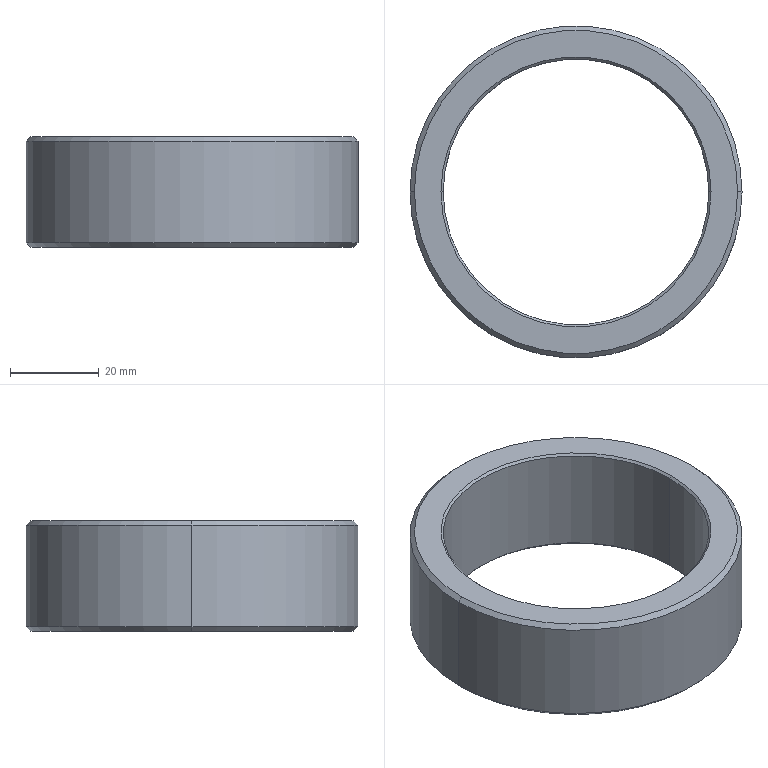Part | SolidWorks | features MBimport 1 | 1 solid | 14 faces | box 75 x 75 x 25 mm | volume 39480 mm3 | cone 8 | cylinder 4 | plane 2 | commonest cylinder face diameters 60 x2 75 x2
STEP:
#1=CARTESIAN_POINT('',(-36.5,0.,-28.514));
#2=VERTEX_POINT('',#1);
#3=CARTESIAN_POINT('',(-37.5,0.,-27.514));
#4=VERTEX_POINT('',#3);
#5=CARTESIAN_POINT('',(-37.5,0.,-27.514));
#6=DIRECTION('',(-0.7071,0.,0.7071));
#7=VECTOR('',#6,1000.);
#8=LINE('',#5,#7);
#9=EDGE_CURVE('',#2,#4,#8,.T.);
#10=ORIENTED_EDGE('',*,*,#9,.F.);
#11=CARTESIAN_POINT('',(36.5,0.,-28.514));
#12=VERTEX_POINT('',#11);
#13=CARTESIAN_POINT('',(0.,0.,-28.514));
#14=DIRECTION('',(0.,0.,-1.));
#15=DIRECTION('',(1.,0.,0.));
#16=AXIS2_PLACEMENT_3D('',#13,#14,#15);
#17=CIRCLE('',#16,36.5);
#18=EDGE_CURVE('',#12,#2,#17,.T.);
#19=ORIENTED_EDGE('',*,*,#18,.F.);
#20=CARTESIAN_POINT('',(37.5,0.,-27.514));
#21=VERTEX_POINT('',#20);
#22=CARTESIAN_POINT('',(37.5,0.,-27.514));
#23=DIRECTION('',(0.7071,0.,0.7071));
#24=VECTOR('',#23,1000.);
#25=LINE('',#22,#24);
#26=EDGE_CURVE('',#12,#21,#25,.T.);
#27=ORIENTED_EDGE('',*,*,#26,.T.);
#28=CARTESIAN_POINT('',(0.,0.,-27.514));
#29=DIRECTION('',(0.,0.,1.));
#30=DIRECTION('',(1.,0.,0.));
#31=AXIS2_PLACEMENT_3D('',#28,#29,#30);
#32=CIRCLE('',#31,37.5);
#33=EDGE_CURVE('',#4,#21,#32,.T.);
#34=ORIENTED_EDGE('',*,*,#33,.F.);
#35=EDGE_LOOP('',(#10,#19,#27,#34));
#36=FACE_OUTER_BOUND('',#35,.T.);
#37=CARTESIAN_POINT('',(0.,0.,-27.514));
#38=DIRECTION('',(0.,0.,1.));
#39=DIRECTION('',(1.,0.,0.));
#40=AXIS2_PLACEMENT_3D('',#37,#38,#39);
#41=CONICAL_SURFACE('',#40,37.5,0.7854);
#42=ADVANCED_FACE('',(#36),#41,.T.);
#43=CARTESIAN_POINT('',(30.,0.,-28.014));
#44=VERTEX_POINT('',#43);
#45=CARTESIAN_POINT('',(30.5,0.,-28.514));
#46=VERTEX_POINT('',#45);
#47=CARTESIAN_POINT('',(30.5,0.,-28.514));
#48=DIRECTION('',(0.7071,0.,-0.7071));
#49=VECTOR('',#48,1000.);
#50=LINE('',#47,#49);
#51=EDGE_CURVE('',#44,#46,#50,.T.);
#52=ORIENTED_EDGE('',*,*,#51,.F.);
#53=CARTESIAN_POINT('',(-30.,0.,-28.014));
#54=VERTEX_POINT('',#53);
#55=CARTESIAN_POINT('',(0.,0.,-28.014));
#56=DIRECTION('',(0.,0.,-1.));
#57=DIRECTION('',(1.,0.,0.));
#58=AXIS2_PLACEMENT_3D('',#55,#56,#57);
#59=CIRCLE('',#58,30.);
#60=EDGE_CURVE('',#54,#44,#59,.T.);
#61=ORIENTED_EDGE('',*,*,#60,.F.);
#62=CARTESIAN_POINT('',(-30.5,0.,-28.514));
#63=VERTEX_POINT('',#62);
#64=CARTESIAN_POINT('',(-30.5,0.,-28.514));
#65=DIRECTION('',(-0.7071,0.,-0.7071));
#66=VECTOR('',#65,1000.);
#67=LINE('',#64,#66);
#68=EDGE_CURVE('',#54,#63,#67,.T.);
#69=ORIENTED_EDGE('',*,*,#68,.T.);
#70=CARTESIAN_POINT('',(0.,0.,-28.514));
#71=DIRECTION('',(0.,0.,1.));
#72=DIRECTION('',(1.,0.,0.));
#73=AXIS2_PLACEMENT_3D('',#70,#71,#72);
#74=CIRCLE('',#73,30.5);
#75=EDGE_CURVE('',#46,#63,#74,.T.);
#76=ORIENTED_EDGE('',*,*,#75,.F.);
#77=EDGE_LOOP('',(#52,#61,#69,#76));
#78=FACE_OUTER_BOUND('',#77,.T.);
#79=CARTESIAN_POINT('',(0.,0.,-28.514));
#80=DIRECTION('',(0.,0.,-1.));
#81=DIRECTION('',(-1.,0.,0.));
#82=AXIS2_PLACEMENT_3D('',#79,#80,#81);
#83=CONICAL_SURFACE('',#82,30.5,0.7854);
#84=ADVANCED_FACE('',(#78),#83,.F.);
#85=CARTESIAN_POINT('',(36.5,0.,-3.514));
#86=VERTEX_POINT('',#85);
#87=CARTESIAN_POINT('',(37.5,0.,-4.514));
#88=VERTEX_POINT('',#87);
#89=CARTESIAN_POINT('',(36.5,0.,-3.514));
#90=DIRECTION('',(0.7071,0.,-0.7071));
#91=VECTOR('',#90,1000.);
#92=LINE('',#89,#91);
#93=EDGE_CURVE('',#86,#88,#92,.T.);
#94=ORIENTED_EDGE('',*,*,#93,.F.);
#95=CARTESIAN_POINT('',(-36.5,0.,-3.514));
#96=VERTEX_POINT('',#95);
#97=CARTESIAN_POINT('',(0.,0.,-3.514));
#98=DIRECTION('',(0.,0.,1.));
#99=DIRECTION('',(-1.,0.,0.));
#100=AXIS2_PLACEMENT_3D('',#97,#98,#99);
#101=CIRCLE('',#100,36.5);
#102=EDGE_CURVE('',#96,#86,#101,.T.);
#103=ORIENTED_EDGE('',*,*,#102,.F.);
#104=CARTESIAN_POINT('',(-37.5,0.,-4.514));
#105=VERTEX_POINT('',#104);
#106=CARTESIAN_POINT('',(-36.5,0.,-3.514));
#107=DIRECTION('',(-0.7071,0.,-0.7071));
#108=VECTOR('',#107,1000.);
#109=LINE('',#106,#108);
#110=EDGE_CURVE('',#96,#105,#109,.T.);
#111=ORIENTED_EDGE('',*,*,#110,.T.);
#112=CARTESIAN_POINT('',(0.,0.,-4.514));
#113=DIRECTION('',(0.,0.,-1.));
#114=DIRECTION('',(-1.,0.,0.));
#115=AXIS2_PLACEMENT_3D('',#112,#113,#114);
#116=CIRCLE('',#115,37.5);
#117=EDGE_CURVE('',#88,#105,#116,.T.);
#118=ORIENTED_EDGE('',*,*,#117,.F.);
#119=EDGE_LOOP('',(#94,#103,#111,#118));
#120=FACE_OUTER_BOUND('',#119,.T.);
#121=CARTESIAN_POINT('',(0.,0.,-3.514));
#122=DIRECTION('',(0.,0.,-1.));
#123=DIRECTION('',(-1.,0.,0.));
#124=AXIS2_PLACEMENT_3D('',#121,#122,#123);
#125=CONICAL_SURFACE('',#124,36.5,0.7854);
#126=ADVANCED_FACE('',(#120),#125,.T.);
#127=CARTESIAN_POINT('',(-30.,0.,-4.014));
#128=VERTEX_POINT('',#127);
#129=CARTESIAN_POINT('',(-30.5,0.,-3.514));
#130=VERTEX_POINT('',#129);
#131=CARTESIAN_POINT('',(-30.,0.,-4.014));
#132=DIRECTION('',(-0.7071,0.,0.7071));
#133=VECTOR('',#132,1000.);
#134=LINE('',#131,#133);
#135=EDGE_CURVE('',#128,#130,#134,.T.);
#136=ORIENTED_EDGE('',*,*,#135,.F.);
#137=CARTESIAN_POINT('',(30.,0.,-4.014));
#138=VERTEX_POINT('',#137);
#139=CARTESIAN_POINT('',(0.,0.,-4.014));
#140=DIRECTION('',(0.,0.,1.));
#141=DIRECTION('',(-1.,0.,0.));
#142=AXIS2_PLACEMENT_3D('',#139,#140,#141);
#143=CIRCLE('',#142,30.);
#144=EDGE_CURVE('',#138,#128,#143,.T.);
#145=ORIENTED_EDGE('',*,*,#144,.F.);
#146=CARTESIAN_POINT('',(30.5,0.,-3.514));
#147=VERTEX_POINT('',#146);
#148=CARTESIAN_POINT('',(30.,0.,-4.014));
#149=DIRECTION('',(0.7071,0.,0.7071));
#150=VECTOR('',#149,1000.);
#151=LINE('',#148,#150);
#152=EDGE_CURVE('',#138,#147,#151,.T.);
#153=ORIENTED_EDGE('',*,*,#152,.T.);
#154=CARTESIAN_POINT('',(0.,0.,-3.514));
#155=DIRECTION('',(0.,0.,-1.));
#156=DIRECTION('',(-1.,0.,0.));
#157=AXIS2_PLACEMENT_3D('',#154,#155,#156);
#158=CIRCLE('',#157,30.5);
#159=EDGE_CURVE('',#130,#147,#158,.T.);
#160=ORIENTED_EDGE('',*,*,#159,.F.);
#161=EDGE_LOOP('',(#136,#145,#153,#160));
#162=FACE_OUTER_BOUND('',#161,.T.);
#163=CARTESIAN_POINT('',(0.,0.,-4.014));
#164=DIRECTION('',(0.,0.,1.));
#165=DIRECTION('',(1.,0.,0.));
#166=AXIS2_PLACEMENT_3D('',#163,#164,#165);
#167=CONICAL_SURFACE('',#166,30.,0.7854);
#168=ADVANCED_FACE('',(#162),#167,.F.);
#169=CARTESIAN_POINT('',(0.,0.,-28.514));
#170=DIRECTION('',(0.,0.,1.));
#171=DIRECTION('',(1.,0.,0.));
#172=AXIS2_PLACEMENT_3D('',#169,#170,#171);
#173=CIRCLE('',#172,30.5);
#174=EDGE_CURVE('',#63,#46,#173,.T.);
#175=ORIENTED_EDGE('',*,*,#174,.T.);
#176=ORIENTED_EDGE('',*,*,#75,.T.);
#177=EDGE_LOOP('',(#175,#176));
#178=FACE_BOUND('',#177,.T.);
#179=ORIENTED_EDGE('',*,*,#18,.T.);
#180=CARTESIAN_POINT('',(0.,0.,-28.514));
#181=DIRECTION('',(0.,0.,-1.));
#182=DIRECTION('',(1.,0.,0.));
#183=AXIS2_PLACEMENT_3D('',#180,#181,#182);
#184=CIRCLE('',#183,36.5);
#185=EDGE_CURVE('',#2,#12,#184,.T.);
#186=ORIENTED_EDGE('',*,*,#185,.T.);
#187=EDGE_LOOP('',(#179,#186));
#188=FACE_OUTER_BOUND('',#187,.T.);
#189=CARTESIAN_POINT('',(-37.5,0.,-28.514));
#190=DIRECTION('',(0.,0.,1.));
#191=DIRECTION('',(1.,0.,0.));
#192=AXIS2_PLACEMENT_3D('',#189,#190,#191);
#193=PLANE('',#192);
#194=ADVANCED_FACE('',(#178,#188),#193,.F.);
#195=CARTESIAN_POINT('',(-30.,0.,0.));
#196=DIRECTION('',(0.,0.,1.));
#197=VECTOR('',#196,1000.);
#198=LINE('',#195,#197);
#199=EDGE_CURVE('',#54,#128,#198,.T.);
#200=ORIENTED_EDGE('',*,*,#199,.F.);
#201=ORIENTED_EDGE('',*,*,#60,.T.);
#202=CARTESIAN_POINT('',(30.,0.,0.));
#203=DIRECTION('',(0.,0.,1.));
#204=VECTOR('',#203,1000.);
#205=LINE('',#202,#204);
#206=EDGE_CURVE('',#44,#138,#205,.T.);
#207=ORIENTED_EDGE('',*,*,#206,.T.);
#208=ORIENTED_EDGE('',*,*,#144,.T.);
#209=EDGE_LOOP('',(#200,#201,#207,#208));
#210=FACE_OUTER_BOUND('',#209,.T.);
#211=CARTESIAN_POINT('',(0.,0.,0.));
#212=DIRECTION('',(0.,0.,1.));
#213=DIRECTION('',(1.,0.,0.));
#214=AXIS2_PLACEMENT_3D('',#211,#212,#213);
#215=CYLINDRICAL_SURFACE('',#214,30.);
#216=ADVANCED_FACE('',(#210),#215,.F.);
#217=CARTESIAN_POINT('',(0.,0.,-3.514));
#218=DIRECTION('',(0.,0.,-1.));
#219=DIRECTION('',(-1.,0.,0.));
#220=AXIS2_PLACEMENT_3D('',#217,#218,#219);
#221=CIRCLE('',#220,30.5);
#222=EDGE_CURVE('',#147,#130,#221,.T.);
#223=ORIENTED_EDGE('',*,*,#222,.T.);
#224=ORIENTED_EDGE('',*,*,#159,.T.);
#225=EDGE_LOOP('',(#223,#224));
#226=FACE_BOUND('',#225,.T.);
#227=ORIENTED_EDGE('',*,*,#102,.T.);
#228=CARTESIAN_POINT('',(0.,0.,-3.514));
#229=DIRECTION('',(0.,0.,1.));
#230=DIRECTION('',(-1.,0.,0.));
#231=AXIS2_PLACEMENT_3D('',#228,#229,#230);
#232=CIRCLE('',#231,36.5);
#233=EDGE_CURVE('',#86,#96,#232,.T.);
#234=ORIENTED_EDGE('',*,*,#233,.T.);
#235=EDGE_LOOP('',(#227,#234));
#236=FACE_OUTER_BOUND('',#235,.T.);
#237=CARTESIAN_POINT('',(-37.5,0.,-3.514));
#238=DIRECTION('',(0.,0.,-1.));
#239=DIRECTION('',(0.,-1.,0.));
#240=AXIS2_PLACEMENT_3D('',#237,#238,#239);
#241=PLANE('',#240);
#242=ADVANCED_FACE('',(#226,#236),#241,.F.);
#243=CARTESIAN_POINT('',(-37.5,0.,0.));
#244=DIRECTION('',(0.,0.,1.));
#245=VECTOR('',#244,1000.);
#246=LINE('',#243,#245);
#247=EDGE_CURVE('',#4,#105,#246,.T.);
#248=ORIENTED_EDGE('',*,*,#247,.F.);
#249=ORIENTED_EDGE('',*,*,#33,.T.);
#250=CARTESIAN_POINT('',(37.5,0.,0.));
#251=DIRECTION('',(0.,0.,1.));
#252=VECTOR('',#251,1000.);
#253=LINE('',#250,#252);
#254=EDGE_CURVE('',#21,#88,#253,.T.);
#255=ORIENTED_EDGE('',*,*,#254,.T.);
#256=ORIENTED_EDGE('',*,*,#117,.T.);
#257=EDGE_LOOP('',(#248,#249,#255,#256));
#258=FACE_OUTER_BOUND('',#257,.T.);
#259=CARTESIAN_POINT('',(0.,0.,0.));
#260=DIRECTION('',(0.,0.,1.));
#261=DIRECTION('',(1.,0.,0.));
#262=AXIS2_PLACEMENT_3D('',#259,#260,#261);
#263=CYLINDRICAL_SURFACE('',#262,37.5);
#264=ADVANCED_FACE('',(#258),#263,.T.);
#265=CARTESIAN_POINT('',(0.,0.,-27.514));
#266=DIRECTION('',(0.,0.,1.));
#267=DIRECTION('',(1.,0.,0.));
#268=AXIS2_PLACEMENT_3D('',#265,#266,#267);
#269=CIRCLE('',#268,37.5);
#270=EDGE_CURVE('',#21,#4,#269,.T.);
#271=ORIENTED_EDGE('',*,*,#270,.T.);
#272=ORIENTED_EDGE('',*,*,#247,.T.);
#273=CARTESIAN_POINT('',(0.,0.,-4.514));
#274=DIRECTION('',(0.,0.,-1.));
#275=DIRECTION('',(-1.,0.,0.));
#276=AXIS2_PLACEMENT_3D('',#273,#274,#275);
#277=CIRCLE('',#276,37.5);
#278=EDGE_CURVE('',#105,#88,#277,.T.);
#279=ORIENTED_EDGE('',*,*,#278,.T.);
#280=ORIENTED_EDGE('',*,*,#254,.F.);
#281=EDGE_LOOP('',(#271,#272,#279,#280));
#282=FACE_OUTER_BOUND('',#281,.T.);
#283=CARTESIAN_POINT('',(0.,0.,0.));
#284=DIRECTION('',(0.,0.,1.));
#285=DIRECTION('',(1.,0.,0.));
#286=AXIS2_PLACEMENT_3D('',#283,#284,#285);
#287=CYLINDRICAL_SURFACE('',#286,37.5);
#288=ADVANCED_FACE('',(#282),#287,.T.);
#289=CARTESIAN_POINT('',(0.,0.,-28.014));
#290=DIRECTION('',(0.,0.,-1.));
#291=DIRECTION('',(1.,0.,0.));
#292=AXIS2_PLACEMENT_3D('',#289,#290,#291);
#293=CIRCLE('',#292,30.);
#294=EDGE_CURVE('',#44,#54,#293,.T.);
#295=ORIENTED_EDGE('',*,*,#294,.T.);
#296=ORIENTED_EDGE('',*,*,#199,.T.);
#297=CARTESIAN_POINT('',(0.,0.,-4.014));
#298=DIRECTION('',(0.,0.,1.));
#299=DIRECTION('',(-1.,0.,0.));
#300=AXIS2_PLACEMENT_3D('',#297,#298,#299);
#301=CIRCLE('',#300,30.);
#302=EDGE_CURVE('',#128,#138,#301,.T.);
#303=ORIENTED_EDGE('',*,*,#302,.T.);
#304=ORIENTED_EDGE('',*,*,#206,.F.);
#305=EDGE_LOOP('',(#295,#296,#303,#304));
#306=FACE_OUTER_BOUND('',#305,.T.);
#307=CARTESIAN_POINT('',(0.,0.,0.));
#308=DIRECTION('',(0.,0.,1.));
#309=DIRECTION('',(1.,0.,0.));
#310=AXIS2_PLACEMENT_3D('',#307,#308,#309);
#311=CYLINDRICAL_SURFACE('',#310,30.);
#312=ADVANCED_FACE('',(#306),#311,.F.);
#313=ORIENTED_EDGE('',*,*,#302,.F.);
#314=ORIENTED_EDGE('',*,*,#135,.T.);
#315=ORIENTED_EDGE('',*,*,#222,.F.);
#316=ORIENTED_EDGE('',*,*,#152,.F.);
#317=EDGE_LOOP('',(#313,#314,#315,#316));
#318=FACE_OUTER_BOUND('',#317,.T.);
#319=CARTESIAN_POINT('',(0.,0.,-4.014));
#320=DIRECTION('',(0.,0.,1.));
#321=DIRECTION('',(1.,0.,0.));
#322=AXIS2_PLACEMENT_3D('',#319,#320,#321);
#323=CONICAL_SURFACE('',#322,30.,0.7854);
#324=ADVANCED_FACE('',(#318),#323,.F.);
#325=ORIENTED_EDGE('',*,*,#233,.F.);
#326=ORIENTED_EDGE('',*,*,#93,.T.);
#327=ORIENTED_EDGE('',*,*,#278,.F.);
#328=ORIENTED_EDGE('',*,*,#110,.F.);
#329=EDGE_LOOP('',(#325,#326,#327,#328));
#330=FACE_OUTER_BOUND('',#329,.T.);
#331=CARTESIAN_POINT('',(0.,0.,-3.514));
#332=DIRECTION('',(0.,0.,-1.));
#333=DIRECTION('',(-1.,0.,0.));
#334=AXIS2_PLACEMENT_3D('',#331,#332,#333);
#335=CONICAL_SURFACE('',#334,36.5,0.7854);
#336=ADVANCED_FACE('',(#330),#335,.T.);
#337=ORIENTED_EDGE('',*,*,#294,.F.);
#338=ORIENTED_EDGE('',*,*,#51,.T.);
#339=ORIENTED_EDGE('',*,*,#174,.F.);
#340=ORIENTED_EDGE('',*,*,#68,.F.);
#341=EDGE_LOOP('',(#337,#338,#339,#340));
#342=FACE_OUTER_BOUND('',#341,.T.);
#343=CARTESIAN_POINT('',(0.,0.,-28.514));
#344=DIRECTION('',(0.,0.,-1.));
#345=DIRECTION('',(-1.,0.,0.));
#346=AXIS2_PLACEMENT_3D('',#343,#344,#345);
#347=CONICAL_SURFACE('',#346,30.5,0.7854);
#348=ADVANCED_FACE('',(#342),#347,.F.);
#349=ORIENTED_EDGE('',*,*,#185,.F.);
#350=ORIENTED_EDGE('',*,*,#9,.T.);
#351=ORIENTED_EDGE('',*,*,#270,.F.);
#352=ORIENTED_EDGE('',*,*,#26,.F.);
#353=EDGE_LOOP('',(#349,#350,#351,#352));
#354=FACE_OUTER_BOUND('',#353,.T.);
#355=CARTESIAN_POINT('',(0.,0.,-27.514));
#356=DIRECTION('',(0.,0.,1.));
#357=DIRECTION('',(1.,0.,0.));
#358=AXIS2_PLACEMENT_3D('',#355,#356,#357);
#359=CONICAL_SURFACE('',#358,37.5,0.7854);
#360=ADVANCED_FACE('',(#354),#359,.T.);
#361=CLOSED_SHELL('',(#42,#84,#126,#168,#194,#216,#242,#264,#288,#312,#324,#336,#348,#360));
#362=MANIFOLD_SOLID_BREP('',#361);
#363=CARTESIAN_POINT('',(0.,0.,0.));
#364=DIRECTION('',(0.,0.,1.));
#365=DIRECTION('',(1.,0.,0.));
#366=AXIS2_PLACEMENT_3D('',#363,#364,#365);
#367=(LENGTH_UNIT()NAMED_UNIT(*)SI_UNIT(.MILLI.,.METRE.));
#368=UNCERTAINTY_MEASURE_WITH_UNIT(LENGTH_MEASURE(0.00001),#367,'','');
#369=(NAMED_UNIT(*)PLANE_ANGLE_UNIT()SI_UNIT($,.RADIAN.));
#370=(NAMED_UNIT(*)SI_UNIT($,.STERADIAN.)SOLID_ANGLE_UNIT());
#371=(GEOMETRIC_REPRESENTATION_CONTEXT(3)GLOBAL_UNCERTAINTY_ASSIGNED_CONTEXT((#368))GLOBAL_UNIT_ASSIGNED_CONTEXT((#367,#369,#370))REPRESENTATION_CONTEXT('',''));
#372=ADVANCED_BREP_SHAPE_REPRESENTATION('',(#362,#366),#371);